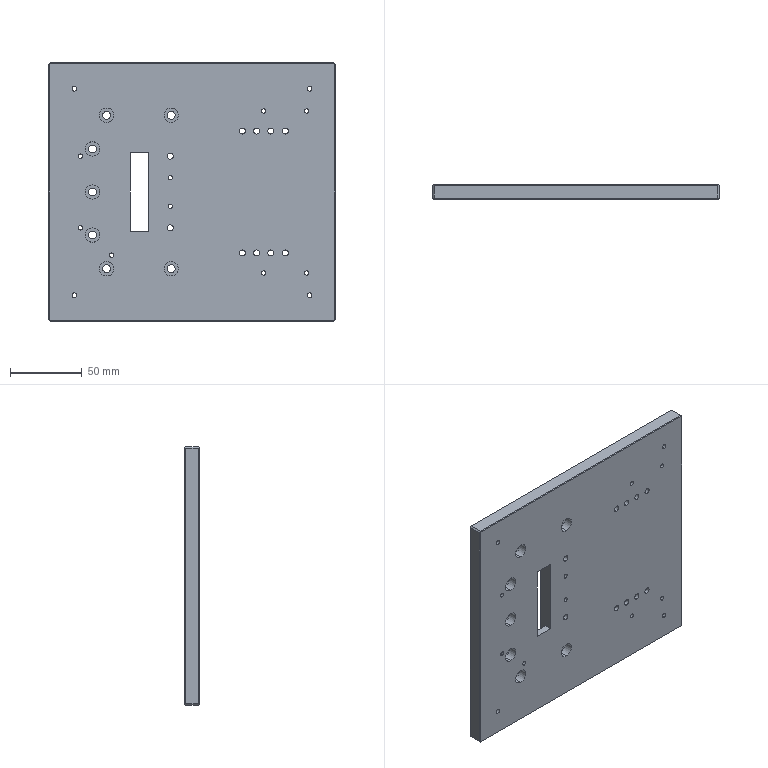Part | SolidWorks | features HoleWzd 6, Chamfer 3, ICE 2, Extrusion 1 | 1 solid | 120 faces | box 200 x 10 x 180 mm | volume 345218 mm3 | cylinder 74 | plane 32 | cone 14 | commonest cylinder face diameters 4.2 x20 3 x18 5.5 x14 10 x14 3.3 x8